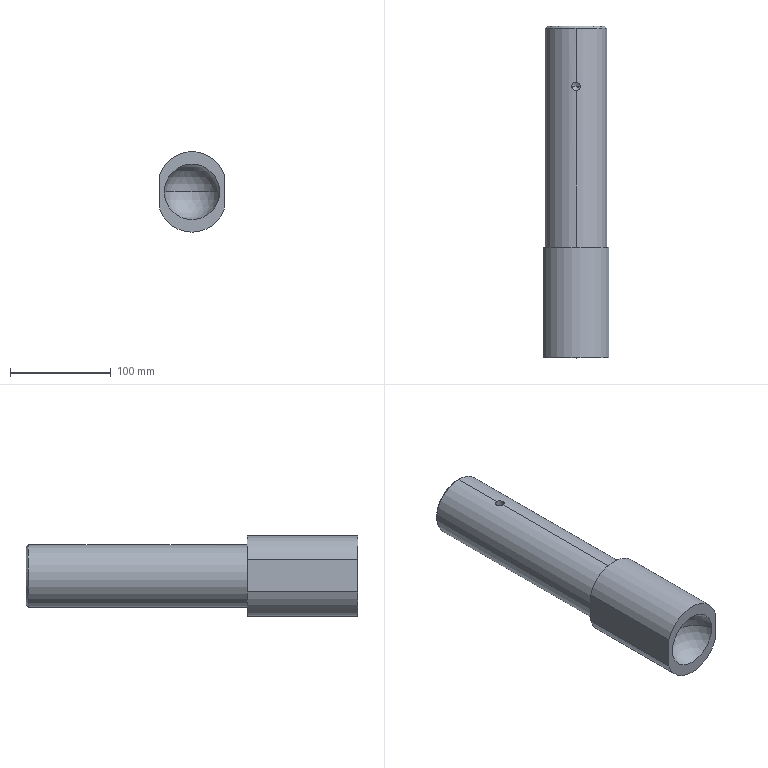Part | SolidWorks | features Chamfer 1, Extrusion 1, HoleWzd 1, ICE 1, RevCut 1 | 1 solid | 18 faces | box 65 x 330 x 80 mm | volume 1109288 mm3 | cylinder 7 | plane 5 | cone 4 | sphere 2 | commonest cylinder face diameters 68 x3 8.5 x2 62 x2
STEP:
#1=CARTESIAN_POINT('',(27.55,0.,0.));
#2=VERTEX_POINT('',#1);
#3=CARTESIAN_POINT('',(-27.55,0.,0.));
#4=VERTEX_POINT('',#3);
#5=CARTESIAN_POINT('',(0.,0.,0.));
#6=DIRECTION('',(0.,-1.,0.));
#7=DIRECTION('',(0.,0.,1.));
#8=AXIS2_PLACEMENT_3D('',#5,#6,#7);
#9=CIRCLE('',#8,27.55);
#10=EDGE_CURVE('',#2,#4,#9,.T.);
#11=ORIENTED_EDGE('',*,*,#10,.T.);
#12=CARTESIAN_POINT('',(0.,23.,0.));
#13=VERTEX_POINT('',#12);
#14=CARTESIAN_POINT('',(0.,-5.,0.));
#15=DIRECTION('',(0.,0.,-1.));
#16=DIRECTION('',(-1.,0.,0.));
#17=AXIS2_PLACEMENT_3D('',#14,#15,#16);
#18=CIRCLE('',#17,28.);
#19=EDGE_CURVE('',#4,#13,#18,.T.);
#20=ORIENTED_EDGE('',*,*,#19,.T.);
#21=CARTESIAN_POINT('',(0.,-5.,0.));
#22=DIRECTION('',(0.,0.,1.));
#23=DIRECTION('',(1.,0.,0.));
#24=AXIS2_PLACEMENT_3D('',#21,#22,#23);
#25=CIRCLE('',#24,28.);
#26=EDGE_CURVE('',#2,#13,#25,.T.);
#27=ORIENTED_EDGE('',*,*,#26,.F.);
#28=EDGE_LOOP('',(#11,#20,#27));
#29=FACE_OUTER_BOUND('',#28,.T.);
#30=CARTESIAN_POINT('',(0.,-5.,0.));
#31=DIRECTION('',(0.,0.,-1.));
#32=DIRECTION('',(1.,0.,0.));
#33=AXIS2_PLACEMENT_3D('',#30,#31,#32);
#34=SPHERICAL_SURFACE('',#33,28.);
#35=ADVANCED_FACE('',(#29),#34,.F.);
#36=CARTESIAN_POINT('',(0.,330.,29.));
#37=VERTEX_POINT('',#36);
#38=CARTESIAN_POINT('',(0.,330.,-29.));
#39=VERTEX_POINT('',#38);
#40=CARTESIAN_POINT('',(0.,330.,0.));
#41=DIRECTION('',(0.,1.,0.));
#42=DIRECTION('',(0.,0.,1.));
#43=AXIS2_PLACEMENT_3D('',#40,#41,#42);
#44=CIRCLE('',#43,29.);
#45=EDGE_CURVE('',#37,#39,#44,.T.);
#46=ORIENTED_EDGE('',*,*,#45,.F.);
#47=CARTESIAN_POINT('',(0.,328.,31.));
#48=VERTEX_POINT('',#47);
#49=CARTESIAN_POINT('',(0.,330.,29.));
#50=DIRECTION('',(0.,-0.7071,0.7071));
#51=VECTOR('',#50,1000.);
#52=LINE('',#49,#51);
#53=EDGE_CURVE('',#37,#48,#52,.T.);
#54=ORIENTED_EDGE('',*,*,#53,.T.);
#55=CARTESIAN_POINT('',(0.,328.,-31.));
#56=VERTEX_POINT('',#55);
#57=CARTESIAN_POINT('',(0.,328.,0.));
#58=DIRECTION('',(0.,-1.,0.));
#59=DIRECTION('',(0.,0.,1.));
#60=AXIS2_PLACEMENT_3D('',#57,#58,#59);
#61=CIRCLE('',#60,31.);
#62=EDGE_CURVE('',#56,#48,#61,.T.);
#63=ORIENTED_EDGE('',*,*,#62,.F.);
#64=CARTESIAN_POINT('',(0.,330.,-29.));
#65=DIRECTION('',(0.,-0.7071,-0.7071));
#66=VECTOR('',#65,1000.);
#67=LINE('',#64,#66);
#68=EDGE_CURVE('',#39,#56,#67,.T.);
#69=ORIENTED_EDGE('',*,*,#68,.F.);
#70=EDGE_LOOP('',(#46,#54,#63,#69));
#71=FACE_OUTER_BOUND('',#70,.T.);
#72=CARTESIAN_POINT('',(0.,330.,0.));
#73=DIRECTION('',(0.,-1.,0.));
#74=DIRECTION('',(0.,0.,-1.));
#75=AXIS2_PLACEMENT_3D('',#72,#73,#74);
#76=CONICAL_SURFACE('',#75,29.,0.7854);
#77=ADVANCED_FACE('',(#71),#76,.T.);
#78=CARTESIAN_POINT('',(0.,270.,0.9463));
#79=VERTEX_POINT('',#78);
#80=CARTESIAN_POINT('',(4.25,270.,3.5));
#81=VERTEX_POINT('',#80);
#82=CARTESIAN_POINT('',(4.25,270.,3.5));
#83=DIRECTION('',(0.8572,0.,0.515));
#84=VECTOR('',#83,1000.);
#85=LINE('',#82,#84);
#86=EDGE_CURVE('',#79,#81,#85,.T.);
#87=ORIENTED_EDGE('',*,*,#86,.F.);
#88=CARTESIAN_POINT('',(-4.25,270.,3.5));
#89=VERTEX_POINT('',#88);
#90=CARTESIAN_POINT('',(-4.25,270.,3.5));
#91=DIRECTION('',(-0.8572,0.,0.515));
#92=VECTOR('',#91,1000.);
#93=LINE('',#90,#92);
#94=EDGE_CURVE('',#79,#89,#93,.T.);
#95=ORIENTED_EDGE('',*,*,#94,.T.);
#96=CARTESIAN_POINT('',(0.,270.,3.5));
#97=DIRECTION('',(0.,0.,1.));
#98=DIRECTION('',(1.,0.,0.));
#99=AXIS2_PLACEMENT_3D('',#96,#97,#98);
#100=CIRCLE('',#99,4.25);
#101=EDGE_CURVE('',#89,#81,#100,.T.);
#102=ORIENTED_EDGE('',*,*,#101,.T.);
#103=EDGE_LOOP('',(#87,#95,#102));
#104=FACE_OUTER_BOUND('',#103,.T.);
#105=CARTESIAN_POINT('',(0.,270.,3.5));
#106=DIRECTION('',(0.,0.,1.));
#107=DIRECTION('',(1.,0.,0.));
#108=AXIS2_PLACEMENT_3D('',#105,#106,#107);
#109=CONICAL_SURFACE('',#108,4.25,1.03);
#110=ADVANCED_FACE('',(#104),#109,.F.);
#111=ORIENTED_EDGE('',*,*,#101,.F.);
#112=CARTESIAN_POINT('',(-4.25,270.,30.707));
#113=VERTEX_POINT('',#112);
#114=CARTESIAN_POINT('',(-4.25,270.,31.));
#115=DIRECTION('',(0.,0.,1.));
#116=VECTOR('',#115,1000.);
#117=LINE('',#114,#116);
#118=EDGE_CURVE('',#89,#113,#117,.T.);
#119=ORIENTED_EDGE('',*,*,#118,.T.);
#120=CARTESIAN_POINT('',(0.,265.75,31.));
#121=VERTEX_POINT('',#120);
#122=CARTESIAN_POINT('',(0.,265.75,31.));
#123=CARTESIAN_POINT('',(-0.2775,265.75,31.));
#124=CARTESIAN_POINT('',(-0.5594,265.778,30.996));
#125=CARTESIAN_POINT('',(-1.105,265.887,30.982));
#126=CARTESIAN_POINT('',(-1.37,265.967,30.971));
#127=CARTESIAN_POINT('',(-1.884,266.18,30.944));
#128=CARTESIAN_POINT('',(-2.133,266.313,30.927));
#129=CARTESIAN_POINT('',(-2.593,266.621,30.892));
#130=CARTESIAN_POINT('',(-2.807,266.797,30.873));
#131=CARTESIAN_POINT('',(-3.204,267.193,30.835));
#132=CARTESIAN_POINT('',(-3.379,267.408,30.816));
#133=CARTESIAN_POINT('',(-3.687,267.868,30.78));
#134=CARTESIAN_POINT('',(-3.82,268.116,30.764));
#135=CARTESIAN_POINT('',(-4.033,268.631,30.737));
#136=CARTESIAN_POINT('',(-4.113,268.895,30.726));
#137=CARTESIAN_POINT('',(-4.222,269.441,30.711));
#138=CARTESIAN_POINT('',(-4.25,269.723,30.707));
#139=CARTESIAN_POINT('',(-4.25,270.,30.707));
#140=B_SPLINE_CURVE_WITH_KNOTS('',3,(#122,#123,#124,#125,#126,#127,#128,#129,#130,#131,#132,#133,#134,#135,#136,#137,#138,#139),.UNSPECIFIED.,.F.,.F.,(4,2,2,2,2,2,2,2,4),(0.006653,0.007484,0.008316,0.009147,0.009978,0.01081,0.01164,0.01247,0.0133),.UNSPECIFIED.);
#141=EDGE_CURVE('',#121,#113,#140,.T.);
#142=ORIENTED_EDGE('',*,*,#141,.F.);
#143=CARTESIAN_POINT('',(4.25,270.,30.707));
#144=VERTEX_POINT('',#143);
#145=CARTESIAN_POINT('',(4.25,270.,30.707));
#146=CARTESIAN_POINT('',(4.25,269.719,30.707));
#147=CARTESIAN_POINT('',(4.222,269.442,30.711));
#148=CARTESIAN_POINT('',(4.114,268.899,30.726));
#149=CARTESIAN_POINT('',(4.032,268.628,30.737));
#150=CARTESIAN_POINT('',(3.819,268.114,30.764));
#151=CARTESIAN_POINT('',(3.688,267.87,30.78));
#152=CARTESIAN_POINT('',(3.379,267.408,30.816));
#153=CARTESIAN_POINT('',(3.2,267.189,30.835));
#154=CARTESIAN_POINT('',(2.808,266.798,30.873));
#155=CARTESIAN_POINT('',(2.594,266.622,30.892));
#156=CARTESIAN_POINT('',(2.13,266.311,30.928));
#157=CARTESIAN_POINT('',(1.883,266.18,30.944));
#158=CARTESIAN_POINT('',(1.371,265.968,30.971));
#159=CARTESIAN_POINT('',(1.103,265.886,30.982));
#160=CARTESIAN_POINT('',(0.5537,265.777,30.996));
#161=CARTESIAN_POINT('',(0.2776,265.75,31.));
#162=CARTESIAN_POINT('',(0.,265.75,31.));
#163=B_SPLINE_CURVE_WITH_KNOTS('',3,(#145,#146,#147,#148,#149,#150,#151,#152,#153,#154,#155,#156,#157,#158,#159,#160,#161,#162),.UNSPECIFIED.,.F.,.F.,(4,2,2,2,2,2,2,2,4),(0.,0.0008316,0.001663,0.002495,0.003327,0.004158,0.00499,0.005821,0.006653),.UNSPECIFIED.);
#164=EDGE_CURVE('',#144,#121,#163,.T.);
#165=ORIENTED_EDGE('',*,*,#164,.F.);
#166=CARTESIAN_POINT('',(4.25,270.,31.));
#167=DIRECTION('',(0.,0.,1.));
#168=VECTOR('',#167,1000.);
#169=LINE('',#166,#168);
#170=EDGE_CURVE('',#81,#144,#169,.T.);
#171=ORIENTED_EDGE('',*,*,#170,.F.);
#172=EDGE_LOOP('',(#111,#119,#142,#165,#171));
#173=FACE_OUTER_BOUND('',#172,.T.);
#174=CARTESIAN_POINT('',(0.,270.,31.));
#175=DIRECTION('',(0.,0.,1.));
#176=DIRECTION('',(1.,0.,0.));
#177=AXIS2_PLACEMENT_3D('',#174,#175,#176);
#178=CYLINDRICAL_SURFACE('',#177,4.25);
#179=ADVANCED_FACE('',(#173),#178,.F.);
#180=ORIENTED_EDGE('',*,*,#62,.T.);
#181=CARTESIAN_POINT('',(0.,274.25,31.));
#182=VERTEX_POINT('',#181);
#183=CARTESIAN_POINT('',(0.,330.,31.));
#184=DIRECTION('',(0.,-1.,0.));
#185=VECTOR('',#184,1000.);
#186=LINE('',#183,#185);
#187=EDGE_CURVE('',#48,#182,#186,.T.);
#188=ORIENTED_EDGE('',*,*,#187,.T.);
#189=CARTESIAN_POINT('',(0.,274.25,31.));
#190=CARTESIAN_POINT('',(0.2808,274.25,31.));
#191=CARTESIAN_POINT('',(0.5569,274.222,30.996));
#192=CARTESIAN_POINT('',(1.1,274.114,30.982));
#193=CARTESIAN_POINT('',(1.371,274.033,30.971));
#194=CARTESIAN_POINT('',(1.885,273.819,30.944));
#195=CARTESIAN_POINT('',(2.128,273.689,30.928));
#196=CARTESIAN_POINT('',(2.59,273.381,30.892));
#197=CARTESIAN_POINT('',(2.808,273.202,30.873));
#198=CARTESIAN_POINT('',(3.2,272.811,30.835));
#199=CARTESIAN_POINT('',(3.376,272.597,30.816));
#200=CARTESIAN_POINT('',(3.687,272.133,30.78));
#201=CARTESIAN_POINT('',(3.818,271.886,30.764));
#202=CARTESIAN_POINT('',(4.031,271.376,30.737));
#203=CARTESIAN_POINT('',(4.113,271.108,30.726));
#204=CARTESIAN_POINT('',(4.222,270.559,30.711));
#205=CARTESIAN_POINT('',(4.25,270.281,30.707));
#206=CARTESIAN_POINT('',(4.25,270.,30.707));
#207=B_SPLINE_CURVE_WITH_KNOTS('',3,(#189,#190,#191,#192,#193,#194,#195,#196,#197,#198,#199,#200,#201,#202,#203,#204,#205,#206),.UNSPECIFIED.,.F.,.F.,(4,2,2,2,2,2,2,2,4),(0.01996,0.02079,0.02162,0.02245,0.02328,0.02411,0.02494,0.02577,0.0266),.UNSPECIFIED.);
#208=EDGE_CURVE('',#182,#144,#207,.T.);
#209=ORIENTED_EDGE('',*,*,#208,.T.);
#210=ORIENTED_EDGE('',*,*,#164,.T.);
#211=CARTESIAN_POINT('',(0.,110.,31.));
#212=VERTEX_POINT('',#211);
#213=CARTESIAN_POINT('',(0.,330.,31.));
#214=DIRECTION('',(0.,-1.,0.));
#215=VECTOR('',#214,1000.);
#216=LINE('',#213,#215);
#217=EDGE_CURVE('',#121,#212,#216,.T.);
#218=ORIENTED_EDGE('',*,*,#217,.T.);
#219=CARTESIAN_POINT('',(0.,110.,-31.));
#220=VERTEX_POINT('',#219);
#221=CARTESIAN_POINT('',(0.,110.,0.));
#222=DIRECTION('',(0.,1.,0.));
#223=DIRECTION('',(0.,0.,1.));
#224=AXIS2_PLACEMENT_3D('',#221,#222,#223);
#225=CIRCLE('',#224,31.);
#226=EDGE_CURVE('',#212,#220,#225,.T.);
#227=ORIENTED_EDGE('',*,*,#226,.T.);
#228=CARTESIAN_POINT('',(0.,330.,-31.));
#229=DIRECTION('',(0.,-1.,0.));
#230=VECTOR('',#229,1000.);
#231=LINE('',#228,#230);
#232=EDGE_CURVE('',#56,#220,#231,.T.);
#233=ORIENTED_EDGE('',*,*,#232,.F.);
#234=EDGE_LOOP('',(#180,#188,#209,#210,#218,#227,#233));
#235=FACE_OUTER_BOUND('',#234,.T.);
#236=CARTESIAN_POINT('',(0.,330.,0.));
#237=DIRECTION('',(0.,-1.,0.));
#238=DIRECTION('',(0.,0.,-1.));
#239=AXIS2_PLACEMENT_3D('',#236,#237,#238);
#240=CYLINDRICAL_SURFACE('',#239,31.);
#241=ADVANCED_FACE('',(#235),#240,.T.);
#242=CARTESIAN_POINT('',(0.,110.,-40.));
#243=VERTEX_POINT('',#242);
#244=CARTESIAN_POINT('',(-32.5,110.,-15.987));
#245=VERTEX_POINT('',#244);
#246=CARTESIAN_POINT('',(0.,110.,-6.));
#247=DIRECTION('',(0.,1.,0.));
#248=DIRECTION('',(0.,0.,1.));
#249=AXIS2_PLACEMENT_3D('',#246,#247,#248);
#250=CIRCLE('',#249,34.);
#251=EDGE_CURVE('',#243,#245,#250,.T.);
#252=ORIENTED_EDGE('',*,*,#251,.F.);
#253=CARTESIAN_POINT('',(0.,0.,-40.));
#254=VERTEX_POINT('',#253);
#255=CARTESIAN_POINT('',(0.,110.,-40.));
#256=DIRECTION('',(0.,-1.,0.));
#257=VECTOR('',#256,1000.);
#258=LINE('',#255,#257);
#259=EDGE_CURVE('',#243,#254,#258,.T.);
#260=ORIENTED_EDGE('',*,*,#259,.T.);
#261=CARTESIAN_POINT('',(-32.5,0.,-15.987));
#262=VERTEX_POINT('',#261);
#263=CARTESIAN_POINT('',(0.,0.,-6.));
#264=DIRECTION('',(0.,1.,0.));
#265=DIRECTION('',(0.,0.,1.));
#266=AXIS2_PLACEMENT_3D('',#263,#264,#265);
#267=CIRCLE('',#266,34.);
#268=EDGE_CURVE('',#254,#262,#267,.T.);
#269=ORIENTED_EDGE('',*,*,#268,.T.);
#270=CARTESIAN_POINT('',(-32.5,110.,-15.987));
#271=DIRECTION('',(0.,-1.,0.));
#272=VECTOR('',#271,1000.);
#273=LINE('',#270,#272);
#274=EDGE_CURVE('',#245,#262,#273,.T.);
#275=ORIENTED_EDGE('',*,*,#274,.F.);
#276=EDGE_LOOP('',(#252,#260,#269,#275));
#277=FACE_OUTER_BOUND('',#276,.T.);
#278=CARTESIAN_POINT('',(0.,110.,-6.));
#279=DIRECTION('',(0.,-1.,0.));
#280=DIRECTION('',(0.,0.,-1.));
#281=AXIS2_PLACEMENT_3D('',#278,#279,#280);
#282=CYLINDRICAL_SURFACE('',#281,34.);
#283=ADVANCED_FACE('',(#277),#282,.T.);
#284=ORIENTED_EDGE('',*,*,#259,.F.);
#285=CARTESIAN_POINT('',(32.5,110.,-15.987));
#286=VERTEX_POINT('',#285);
#287=CARTESIAN_POINT('',(0.,110.,-6.));
#288=DIRECTION('',(0.,1.,0.));
#289=DIRECTION('',(0.,0.,1.));
#290=AXIS2_PLACEMENT_3D('',#287,#288,#289);
#291=CIRCLE('',#290,34.);
#292=EDGE_CURVE('',#286,#243,#291,.T.);
#293=ORIENTED_EDGE('',*,*,#292,.F.);
#294=CARTESIAN_POINT('',(32.5,0.,-15.987));
#295=VERTEX_POINT('',#294);
#296=CARTESIAN_POINT('',(32.5,110.,-15.987));
#297=DIRECTION('',(0.,-1.,0.));
#298=VECTOR('',#297,1000.);
#299=LINE('',#296,#298);
#300=EDGE_CURVE('',#286,#295,#299,.T.);
#301=ORIENTED_EDGE('',*,*,#300,.T.);
#302=CARTESIAN_POINT('',(0.,0.,-6.));
#303=DIRECTION('',(0.,1.,0.));
#304=DIRECTION('',(0.,0.,1.));
#305=AXIS2_PLACEMENT_3D('',#302,#303,#304);
#306=CIRCLE('',#305,34.);
#307=EDGE_CURVE('',#295,#254,#306,.T.);
#308=ORIENTED_EDGE('',*,*,#307,.T.);
#309=EDGE_LOOP('',(#284,#293,#301,#308));
#310=FACE_OUTER_BOUND('',#309,.T.);
#311=CARTESIAN_POINT('',(0.,110.,-6.));
#312=DIRECTION('',(0.,-1.,0.));
#313=DIRECTION('',(0.,0.,-1.));
#314=AXIS2_PLACEMENT_3D('',#311,#312,#313);
#315=CYLINDRICAL_SURFACE('',#314,34.);
#316=ADVANCED_FACE('',(#310),#315,.T.);
#317=CARTESIAN_POINT('',(-32.5,0.,15.987));
#318=VERTEX_POINT('',#317);
#319=CARTESIAN_POINT('',(-32.5,0.,15.987));
#320=DIRECTION('',(0.,0.,1.));
#321=VECTOR('',#320,1000.);
#322=LINE('',#319,#321);
#323=EDGE_CURVE('',#262,#318,#322,.T.);
#324=ORIENTED_EDGE('',*,*,#323,.T.);
#325=CARTESIAN_POINT('',(-32.5,110.,15.987));
#326=VERTEX_POINT('',#325);
#327=CARTESIAN_POINT('',(-32.5,110.,15.987));
#328=DIRECTION('',(0.,-1.,0.));
#329=VECTOR('',#328,1000.);
#330=LINE('',#327,#329);
#331=EDGE_CURVE('',#326,#318,#330,.T.);
#332=ORIENTED_EDGE('',*,*,#331,.F.);
#333=CARTESIAN_POINT('',(-32.5,110.,15.987));
#334=DIRECTION('',(0.,0.,1.));
#335=VECTOR('',#334,1000.);
#336=LINE('',#333,#335);
#337=EDGE_CURVE('',#245,#326,#336,.T.);
#338=ORIENTED_EDGE('',*,*,#337,.F.);
#339=ORIENTED_EDGE('',*,*,#274,.T.);
#340=EDGE_LOOP('',(#324,#332,#338,#339));
#341=FACE_OUTER_BOUND('',#340,.T.);
#342=CARTESIAN_POINT('',(-32.5,110.,15.987));
#343=DIRECTION('',(1.,0.,0.));
#344=DIRECTION('',(0.,0.,-1.));
#345=AXIS2_PLACEMENT_3D('',#342,#343,#344);
#346=PLANE('',#345);
#347=ADVANCED_FACE('',(#341),#346,.F.);
#348=CARTESIAN_POINT('',(32.5,0.,15.987));
#349=VERTEX_POINT('',#348);
#350=CARTESIAN_POINT('',(0.,0.,6.));
#351=DIRECTION('',(0.,1.,0.));
#352=DIRECTION('',(0.,0.,-1.));
#353=AXIS2_PLACEMENT_3D('',#350,#351,#352);
#354=CIRCLE('',#353,34.);
#355=EDGE_CURVE('',#318,#349,#354,.T.);
#356=ORIENTED_EDGE('',*,*,#355,.T.);
#357=CARTESIAN_POINT('',(32.5,110.,15.987));
#358=VERTEX_POINT('',#357);
#359=CARTESIAN_POINT('',(32.5,110.,15.987));
#360=DIRECTION('',(0.,-1.,0.));
#361=VECTOR('',#360,1000.);
#362=LINE('',#359,#361);
#363=EDGE_CURVE('',#358,#349,#362,.T.);
#364=ORIENTED_EDGE('',*,*,#363,.F.);
#365=CARTESIAN_POINT('',(0.,110.,6.));
#366=DIRECTION('',(0.,1.,0.));
#367=DIRECTION('',(0.,0.,-1.));
#368=AXIS2_PLACEMENT_3D('',#365,#366,#367);
#369=CIRCLE('',#368,34.);
#370=EDGE_CURVE('',#326,#358,#369,.T.);
#371=ORIENTED_EDGE('',*,*,#370,.F.);
#372=ORIENTED_EDGE('',*,*,#331,.T.);
#373=EDGE_LOOP('',(#356,#364,#371,#372));
#374=FACE_OUTER_BOUND('',#373,.T.);
#375=CARTESIAN_POINT('',(0.,110.,6.));
#376=DIRECTION('',(0.,-1.,0.));
#377=DIRECTION('',(0.,0.,-1.));
#378=AXIS2_PLACEMENT_3D('',#375,#376,#377);
#379=CYLINDRICAL_SURFACE('',#378,34.);
#380=ADVANCED_FACE('',(#374),#379,.T.);
#381=CARTESIAN_POINT('',(32.5,0.,15.987));
#382=DIRECTION('',(0.,0.,-1.));
#383=VECTOR('',#382,1000.);
#384=LINE('',#381,#383);
#385=EDGE_CURVE('',#349,#295,#384,.T.);
#386=ORIENTED_EDGE('',*,*,#385,.T.);
#387=ORIENTED_EDGE('',*,*,#300,.F.);
#388=CARTESIAN_POINT('',(32.5,110.,15.987));
#389=DIRECTION('',(0.,0.,-1.));
#390=VECTOR('',#389,1000.);
#391=LINE('',#388,#390);
#392=EDGE_CURVE('',#358,#286,#391,.T.);
#393=ORIENTED_EDGE('',*,*,#392,.F.);
#394=ORIENTED_EDGE('',*,*,#363,.T.);
#395=EDGE_LOOP('',(#386,#387,#393,#394));
#396=FACE_OUTER_BOUND('',#395,.T.);
#397=CARTESIAN_POINT('',(32.5,110.,15.987));
#398=DIRECTION('',(-1.,0.,0.));
#399=DIRECTION('',(0.,0.,1.));
#400=AXIS2_PLACEMENT_3D('',#397,#398,#399);
#401=PLANE('',#400);
#402=ADVANCED_FACE('',(#396),#401,.F.);
#403=CARTESIAN_POINT('',(0.,110.,0.));
#404=DIRECTION('',(0.,1.,0.));
#405=DIRECTION('',(0.,0.,1.));
#406=AXIS2_PLACEMENT_3D('',#403,#404,#405);
#407=CIRCLE('',#406,31.);
#408=EDGE_CURVE('',#220,#212,#407,.T.);
#409=ORIENTED_EDGE('',*,*,#408,.F.);
#410=ORIENTED_EDGE('',*,*,#226,.F.);
#411=EDGE_LOOP('',(#409,#410));
#412=FACE_BOUND('',#411,.T.);
#413=ORIENTED_EDGE('',*,*,#292,.T.);
#414=ORIENTED_EDGE('',*,*,#251,.T.);
#415=ORIENTED_EDGE('',*,*,#337,.T.);
#416=ORIENTED_EDGE('',*,*,#370,.T.);
#417=ORIENTED_EDGE('',*,*,#392,.T.);
#418=EDGE_LOOP('',(#413,#414,#415,#416,#417));
#419=FACE_OUTER_BOUND('',#418,.T.);
#420=CARTESIAN_POINT('',(0.,110.,-6.));
#421=DIRECTION('',(0.,1.,0.));
#422=DIRECTION('',(0.,0.,1.));
#423=AXIS2_PLACEMENT_3D('',#420,#421,#422);
#424=PLANE('',#423);
#425=ADVANCED_FACE('',(#412,#419),#424,.T.);
#426=ORIENTED_EDGE('',*,*,#10,.F.);
#427=CARTESIAN_POINT('',(0.,0.,0.));
#428=DIRECTION('',(0.,-1.,0.));
#429=DIRECTION('',(0.,0.,1.));
#430=AXIS2_PLACEMENT_3D('',#427,#428,#429);
#431=CIRCLE('',#430,27.55);
#432=EDGE_CURVE('',#4,#2,#431,.T.);
#433=ORIENTED_EDGE('',*,*,#432,.F.);
#434=EDGE_LOOP('',(#426,#433));
#435=FACE_BOUND('',#434,.T.);
#436=ORIENTED_EDGE('',*,*,#307,.F.);
#437=ORIENTED_EDGE('',*,*,#385,.F.);
#438=ORIENTED_EDGE('',*,*,#355,.F.);
#439=ORIENTED_EDGE('',*,*,#323,.F.);
#440=ORIENTED_EDGE('',*,*,#268,.F.);
#441=EDGE_LOOP('',(#436,#437,#438,#439,#440));
#442=FACE_OUTER_BOUND('',#441,.T.);
#443=CARTESIAN_POINT('',(0.,0.,-6.));
#444=DIRECTION('',(0.,1.,0.));
#445=DIRECTION('',(0.,0.,1.));
#446=AXIS2_PLACEMENT_3D('',#443,#444,#445);
#447=PLANE('',#446);
#448=ADVANCED_FACE('',(#435,#442),#447,.F.);
#449=ORIENTED_EDGE('',*,*,#187,.F.);
#450=CARTESIAN_POINT('',(0.,328.,0.));
#451=DIRECTION('',(0.,-1.,0.));
#452=DIRECTION('',(0.,0.,1.));
#453=AXIS2_PLACEMENT_3D('',#450,#451,#452);
#454=CIRCLE('',#453,31.);
#455=EDGE_CURVE('',#48,#56,#454,.T.);
#456=ORIENTED_EDGE('',*,*,#455,.T.);
#457=ORIENTED_EDGE('',*,*,#232,.T.);
#458=ORIENTED_EDGE('',*,*,#408,.T.);
#459=ORIENTED_EDGE('',*,*,#217,.F.);
#460=ORIENTED_EDGE('',*,*,#141,.T.);
#461=CARTESIAN_POINT('',(-4.25,270.,30.707));
#462=CARTESIAN_POINT('',(-4.25,270.278,30.707));
#463=CARTESIAN_POINT('',(-4.223,270.554,30.711));
#464=CARTESIAN_POINT('',(-4.114,271.103,30.726));
#465=CARTESIAN_POINT('',(-4.032,271.371,30.737));
#466=CARTESIAN_POINT('',(-3.82,271.883,30.764));
#467=CARTESIAN_POINT('',(-3.688,272.13,30.78));
#468=CARTESIAN_POINT('',(-3.378,272.594,30.816));
#469=CARTESIAN_POINT('',(-3.202,272.808,30.835));
#470=CARTESIAN_POINT('',(-2.81,273.2,30.873));
#471=CARTESIAN_POINT('',(-2.592,273.38,30.892));
#472=CARTESIAN_POINT('',(-2.13,273.688,30.928));
#473=CARTESIAN_POINT('',(-1.886,273.819,30.944));
#474=CARTESIAN_POINT('',(-1.371,274.032,30.971));
#475=CARTESIAN_POINT('',(-1.102,274.114,30.982));
#476=CARTESIAN_POINT('',(-0.5579,274.222,30.996));
#477=CARTESIAN_POINT('',(-0.281,274.25,31.));
#478=CARTESIAN_POINT('',(0.,274.25,31.));
#479=B_SPLINE_CURVE_WITH_KNOTS('',3,(#461,#462,#463,#464,#465,#466,#467,#468,#469,#470,#471,#472,#473,#474,#475,#476,#477,#478),.UNSPECIFIED.,.F.,.F.,(4,2,2,2,2,2,2,2,4),(0.0133,0.01413,0.01497,0.0158,0.01663,0.01746,0.01829,0.01912,0.01996),.UNSPECIFIED.);
#480=EDGE_CURVE('',#113,#182,#479,.T.);
#481=ORIENTED_EDGE('',*,*,#480,.T.);
#482=EDGE_LOOP('',(#449,#456,#457,#458,#459,#460,#481));
#483=FACE_OUTER_BOUND('',#482,.T.);
#484=CARTESIAN_POINT('',(0.,330.,0.));
#485=DIRECTION('',(0.,-1.,0.));
#486=DIRECTION('',(0.,0.,-1.));
#487=AXIS2_PLACEMENT_3D('',#484,#485,#486);
#488=CYLINDRICAL_SURFACE('',#487,31.);
#489=ADVANCED_FACE('',(#483),#488,.T.);
#490=CARTESIAN_POINT('',(0.,330.,0.));
#491=DIRECTION('',(0.,1.,0.));
#492=DIRECTION('',(0.,0.,1.));
#493=AXIS2_PLACEMENT_3D('',#490,#491,#492);
#494=CIRCLE('',#493,29.);
#495=EDGE_CURVE('',#39,#37,#494,.T.);
#496=ORIENTED_EDGE('',*,*,#495,.T.);
#497=ORIENTED_EDGE('',*,*,#45,.T.);
#498=EDGE_LOOP('',(#496,#497));
#499=FACE_OUTER_BOUND('',#498,.T.);
#500=CARTESIAN_POINT('',(0.,330.,0.));
#501=DIRECTION('',(0.,1.,0.));
#502=DIRECTION('',(0.,0.,1.));
#503=AXIS2_PLACEMENT_3D('',#500,#501,#502);
#504=PLANE('',#503);
#505=ADVANCED_FACE('',(#499),#504,.T.);
#506=ORIENTED_EDGE('',*,*,#118,.F.);
#507=CARTESIAN_POINT('',(0.,270.,3.5));
#508=DIRECTION('',(0.,0.,1.));
#509=DIRECTION('',(1.,0.,0.));
#510=AXIS2_PLACEMENT_3D('',#507,#508,#509);
#511=CIRCLE('',#510,4.25);
#512=EDGE_CURVE('',#81,#89,#511,.T.);
#513=ORIENTED_EDGE('',*,*,#512,.F.);
#514=ORIENTED_EDGE('',*,*,#170,.T.);
#515=ORIENTED_EDGE('',*,*,#208,.F.);
#516=ORIENTED_EDGE('',*,*,#480,.F.);
#517=EDGE_LOOP('',(#506,#513,#514,#515,#516));
#518=FACE_OUTER_BOUND('',#517,.T.);
#519=CARTESIAN_POINT('',(0.,270.,31.));
#520=DIRECTION('',(0.,0.,1.));
#521=DIRECTION('',(1.,0.,0.));
#522=AXIS2_PLACEMENT_3D('',#519,#520,#521);
#523=CYLINDRICAL_SURFACE('',#522,4.25);
#524=ADVANCED_FACE('',(#518),#523,.F.);
#525=ORIENTED_EDGE('',*,*,#94,.F.);
#526=ORIENTED_EDGE('',*,*,#86,.T.);
#527=ORIENTED_EDGE('',*,*,#512,.T.);
#528=EDGE_LOOP('',(#525,#526,#527));
#529=FACE_OUTER_BOUND('',#528,.T.);
#530=CARTESIAN_POINT('',(0.,270.,3.5));
#531=DIRECTION('',(0.,0.,1.));
#532=DIRECTION('',(1.,0.,0.));
#533=AXIS2_PLACEMENT_3D('',#530,#531,#532);
#534=CONICAL_SURFACE('',#533,4.25,1.03);
#535=ADVANCED_FACE('',(#529),#534,.F.);
#536=ORIENTED_EDGE('',*,*,#53,.F.);
#537=ORIENTED_EDGE('',*,*,#495,.F.);
#538=ORIENTED_EDGE('',*,*,#68,.T.);
#539=ORIENTED_EDGE('',*,*,#455,.F.);
#540=EDGE_LOOP('',(#536,#537,#538,#539));
#541=FACE_OUTER_BOUND('',#540,.T.);
#542=CARTESIAN_POINT('',(0.,330.,0.));
#543=DIRECTION('',(0.,-1.,0.));
#544=DIRECTION('',(0.,0.,-1.));
#545=AXIS2_PLACEMENT_3D('',#542,#543,#544);
#546=CONICAL_SURFACE('',#545,29.,0.7854);
#547=ADVANCED_FACE('',(#541),#546,.T.);
#548=ORIENTED_EDGE('',*,*,#19,.F.);
#549=ORIENTED_EDGE('',*,*,#432,.T.);
#550=ORIENTED_EDGE('',*,*,#26,.T.);
#551=EDGE_LOOP('',(#548,#549,#550));
#552=FACE_OUTER_BOUND('',#551,.T.);
#553=CARTESIAN_POINT('',(0.,-5.,0.));
#554=DIRECTION('',(0.,0.,-1.));
#555=DIRECTION('',(1.,0.,0.));
#556=AXIS2_PLACEMENT_3D('',#553,#554,#555);
#557=SPHERICAL_SURFACE('',#556,28.);
#558=ADVANCED_FACE('',(#552),#557,.F.);
#559=CLOSED_SHELL('',(#35,#77,#110,#179,#241,#283,#316,#347,#380,#402,#425,#448,#489,#505,#524,#535,#547,#558));
#560=MANIFOLD_SOLID_BREP('',#559);
#561=CARTESIAN_POINT('',(0.,0.,0.));
#562=DIRECTION('',(0.,0.,1.));
#563=DIRECTION('',(1.,0.,0.));
#564=AXIS2_PLACEMENT_3D('',#561,#562,#563);
#565=(LENGTH_UNIT()NAMED_UNIT(*)SI_UNIT(.MILLI.,.METRE.));
#566=UNCERTAINTY_MEASURE_WITH_UNIT(LENGTH_MEASURE(0.00001),#565,'','');
#567=(NAMED_UNIT(*)PLANE_ANGLE_UNIT()SI_UNIT($,.RADIAN.));
#568=(NAMED_UNIT(*)SI_UNIT($,.STERADIAN.)SOLID_ANGLE_UNIT());
#569=(GEOMETRIC_REPRESENTATION_CONTEXT(3)GLOBAL_UNCERTAINTY_ASSIGNED_CONTEXT((#566))GLOBAL_UNIT_ASSIGNED_CONTEXT((#565,#567,#568))REPRESENTATION_CONTEXT('',''));
#570=ADVANCED_BREP_SHAPE_REPRESENTATION('',(#560,#564),#569);